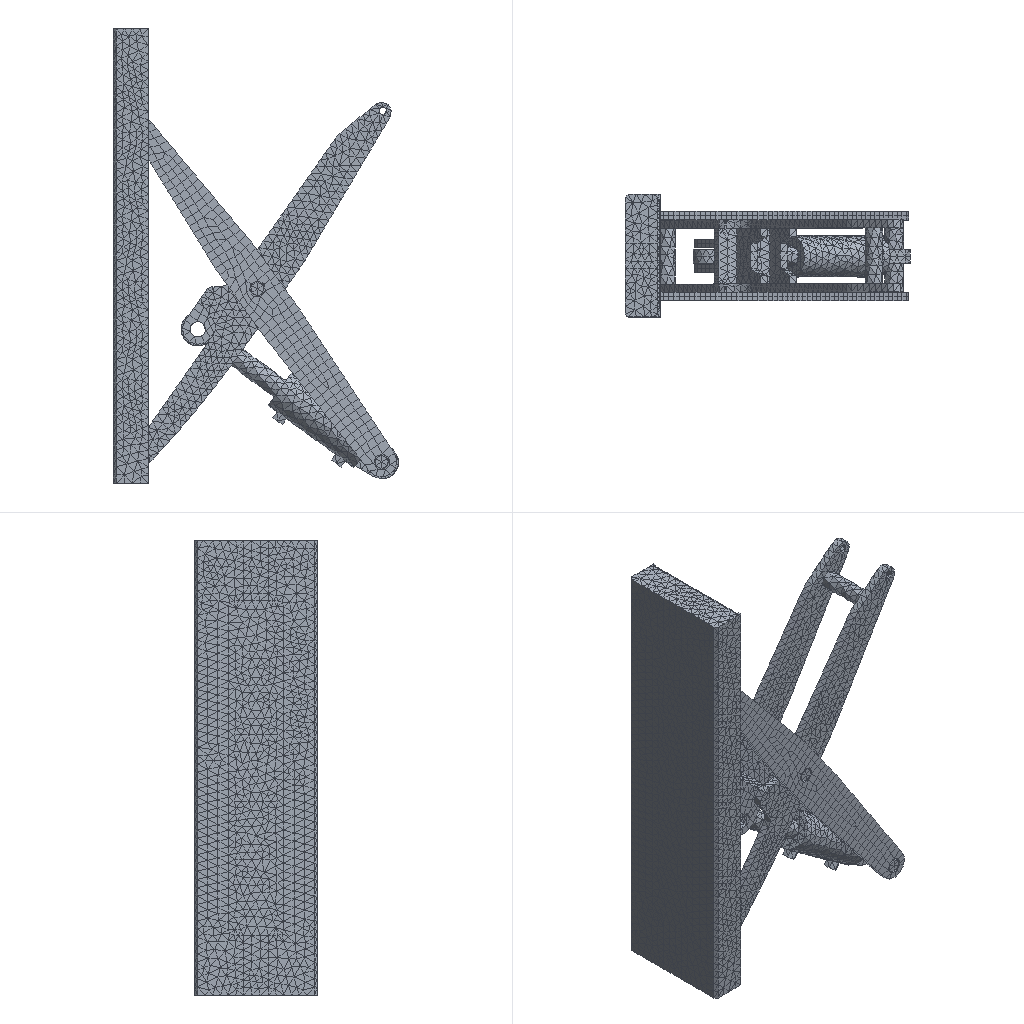Simulation study | ansys workbench
Set-up summary:
category,name,step,type,value,unit,region
solver,ansys_mapdl
solver,version,,,20.2
units,MPA,,stated
analysis,deck,,transient,transient
load_step,requested,,,2
analysis,nlgeom,,,True
mesh,nodes,,,10198
mesh,elements,,,28619
element_type,ANSYS 185 (type 1),,solid,12454
element_type,ANSYS 185 (type 2),,solid,5961
element_type,ANSYS 185 (type 3),,solid,52
element_type,ANSYS 185 (type 4),,solid,52
element_type,ANSYS 185 (type 5),,solid,490
element_type,ANSYS 185 (type 6),,solid,490
element_type,ANSYS 185 (type 7),,solid,1736
element_type,ANSYS 185 (type 8),,solid,725
element_type,ANSYS 185 (type 9),,solid,425
element_type,ANSYS 185 (type 10),,solid,1992
element_type,ANSYS 185 (type 11),,solid,1163
element_type,ANSYS 154 (type 12),,surface,706
element_type,ANSYS 174 (type 13),,contact,30
element_type,ANSYS 170 (type 14),,target,0
element_type,ANSYS 174 (type 15),,contact,12
element_type,ANSYS 170 (type 16),,target,0
element_type,ANSYS 174 (type 17),,contact,50
element_type,ANSYS 170 (type 18),,target,0
element_type,ANSYS 174 (type 19),,contact,12
element_type,ANSYS 170 (type 20),,target,0
element_type,ANSYS 174 (type 21),,contact,20
element_type,ANSYS 170 (type 22),,target,0
element_type,ANSYS 174 (type 23),,contact,12
element_type,ANSYS 170 (type 24),,target,0
element_type,ANSYS 174 (type 25),,contact,20
element_type,ANSYS 170 (type 26),,target,0
element_type,ANSYS 174 (type 27),,contact,12
element_type,ANSYS 170 (type 28),,target,0
element_type,ANSYS 174 (type 29),,contact,20
element_type,ANSYS 170 (type 30),,target,0
element_type,ANSYS 174 (type 31),,contact,14
element_type,ANSYS 170 (type 32),,target,0
element_type,ANSYS 174 (type 33),,contact,20
element_type,ANSYS 170 (type 34),,target,0
element_type,ANSYS 174 (type 35),,contact,14
element_type,ANSYS 170 (type 36),,target,0
element_type,ANSYS 174 (type 37),,contact,22
element_type,ANSYS 170 (type 38),,target,0
element_type,ANSYS 174 (type 39),,contact,14
element_type,ANSYS 170 (type 40),,target,0
element_type,ANSYS 174 (type 41),,contact,22
element_type,ANSYS 170 (type 42),,target,0
element_type,ANSYS 174 (type 43),,contact,14
element_type,ANSYS 170 (type 44),,target,0
element_type,ANSYS 174 (type 45),,contact,24
element_type,ANSYS 170 (type 46),,target,0
element_type,ANSYS 174 (type 47),,contact,28
element_type,ANSYS 170 (type 48),,target,0
element_type,ANSYS 174 (type 49),,contact,52
element_type,ANSYS 170 (type 50),,target,0
element_type,ANSYS 174 (type 51),,contact,334
element_type,ANSYS 170 (type 52),,target,0
element_type,ANSYS 174 (type 53),,contact,32
element_type,ANSYS 170 (type 54),,target,0
element_type,ANSYS 174 (type 55),,contact,56
element_type,ANSYS 170 (type 56),,target,0
element_type,ANSYS 174 (type 57),,contact,104
element_type,ANSYS 170 (type 58),,target,0
element_type,ANSYS 174 (type 59),,contact,56
element_type,ANSYS 170 (type 60),,target,0
element_type,ANSYS 174 (type 61),,contact,116
element_type,ANSYS 170 (type 62),,target,0
element_type,ANSYS 174 (type 63),,contact,1037
element_type,ANSYS 170 (type 64),,target,0
element_type,ANSYS 174 (type 65),,contact,32
element_type,ANSYS 170 (type 66),,target,0
element_type,ANSYS 174 (type 67),,contact,122
element_type,ANSYS 170 (type 68),,target,0
element_type,ANSYS 174 (type 69),,contact,28
element_type,ANSYS 170 (type 70),,target,0
element_type,ANSYS 174 (type 71),,contact,28
element_type,ANSYS 170 (type 72),,target,0
element_type,ANSYS 184 (type 73),,mpc,1
element_type,ANSYS 184 (type 74),,mpc,1
element_type,ANSYS 184 (type 75),,mpc,1
element_type,ANSYS 184 (type 76),,mpc,1
element_type,ANSYS 184 (type 77),,mpc,1
element_type,ANSYS 184 (type 78),,mpc,1
element_type,ANSYS 184 (type 79),,mpc,1
element_type,ANSYS 184 (type 80),,mpc,1
element_type,ANSYS 184 (type 81),,mpc,1
element_type,ANSYS 184 (type 82),,mpc,1
element_type,ANSYS 184 (type 83),,mpc,1
element_type,ANSYS 184 (type 84),,mpc,1
element_type,ANSYS 184 (type 85),,mpc,1
element_type,ANSYS 184 (type 86),,mpc,1
element_type,ANSYS 184 (type 87),,mpc,1
element_type,ANSYS 184 (type 88),,mpc,1
load,load commands in deck,,count,4
bc,support commands in deck,,count,1
named_set,_ELMISC,,component
material,1,,in results
material,2,,in results
material,3,,in results
material,4,,in results
material,5,,in results
material,6,,in results
material,7,,in results
material,8,,in results
material,9,,in results
material,10,,in results
material,11,,in results
check,setup vs results,,match,"results also hold 0 node(s) and 30 element(s) the deck makes with ['EN']; those were not compared; 2 setup node(s) no element uses are not in the results (e.g. [10272, 10274]); 78 node(s) the solver created internally for pilot nodes (solve.out) are in the results only; 706 surface effect element(s) are not in the reader's mesh and were not compared"
Ansys APDL input file, long lists of numbers shortened:
/batch
/config,noeldb,1     ! force off writing results to database
*get,_wallstrt,active,,time,wall
! ANSYS input file written by Workbench version 2020 R2
! File used for geometry attach: E:\LINSHIWENJIAN\WB_DESKTOP-V417B2O_Adminis_37620_2\unsaved_project_files\dp0\Geom\DM\Geom.scdoc
/title,___st--__ (B5)
*DIM,_wb_ProjectScratch_dir,string,248
_wb_ProjectScratch_dir(1) = 'E:\_ProjectScratch\ScrF0D5\'
*DIM,_wb_SolverFiles_dir,string,248
_wb_SolverFiles_dir(1) = 'E:\升降台st_files\dp0\SYS-1\MECH\'
*DIM,_wb_userfiles_dir,string,248
_wb_userfiles_dir(1) = 'E:\升降台st_files\user_files\'
/com,--- Data in consistent NMM units. See Solving Units in the help system for more information.
/units,MPA
/nopr
/wb,file,start              !  signify a WB generated input file
/prep7
! Turn off shape checking because checks already performed inside WB mesher.
! See help system for more information.
SHPP,OFF,,NOWARN
/nolist
etcon,set             ! allow ANSYS to choose best KEYOP's for 180x elements
/com,*********** Nodes for the whole assembly ***********
nblock,3,,11182
(1i9,3e20.9e3)
        1    -5.667923198E+02    -1.150000000E+02     5.191691898E+02
! (10165 more lines like these left out)
-1
/com,*********** Nodes for all Remote Points ***********
nblock,3
(1i9,3e20.9e3)
    10244    -8.508159903E+02    -3.149998116E+01     1.243113147E+03
! (31 more lines like these left out)
-1
/wb,elem,start            !  set before creation of elements
/com,*********** Elements for Body 1 "____\____5" ***********
et,1,185
eblock,19,solid,,12454
(19i9)
        1        1        1        1        0        0        0        0        8        0    12107     5574     8263     8237     8237     8258     8258     8258     8258
! (12453 more lines like these left out)
-1
/com,*********** Elements for Body 2 "______1\____-____9" ***********
et,2,185
eblock,19,solid,,5961
(19i9)
        2        2        2        2        0        0        0        0        8        0     6146     2654     2655     2896     2896     4170     4170     4170     4170
! (5960 more lines like these left out)
-1
/com,*********** Elements for Body 3 "______1\____-____4[2]" ***********
et,3,185
eblock,19,solid,,52
(19i9)
        3        3        3        3        0        0        0        0        8        0     3377     1207     1213     1269     1268     1220     1214     1277     1276
! (51 more lines like these left out)
-1
/com,*********** Elements for Body 4 "______1\____-____4[1]" ***********
et,4,185
eblock,19,solid,,52
(19i9)
        4        4        4        4        0        0        0        0        8        0        1        3        9       65       64       16       10       69       70
! (51 more lines like these left out)
-1
/com,*********** Elements for Body 5 "______2-2\____-____1" ***********
et,5,185
eblock,19,solid,,490
(19i9)
        5        5        5        5        0        0        0        0        8        0    24561     8325     8494     8376     8483     8670     8501     8619     8512
! (489 more lines like these left out)
-1
/com,*********** Elements for Body 6 "______2-2\____-____1" ***********
et,6,185
eblock,19,solid,,490
(19i9)
        6        6        6        6        0        0        0        0        8        0    25051     9246     9415     9297     9404     9591     9422     9540     9433
! (489 more lines like these left out)
-1
/com,*********** Elements for Body 7 "________\M27 ______1" ***********
et,7,185
eblock,19,solid,,1736
(19i9)
        7        7        7        7        0        0        0        0        8        0      478      387      466      865      865      859      859      859      859
! (1735 more lines like these left out)
-1
/com,*********** Elements for Body 8 "________-4\____-____4" ***********
et,8,185
eblock,19,solid,,725
(19i9)
        8        8        8        8        0        0        0        0        8        0     3429     1336     1516     1518     1518     1576     1576     1576     1576
! (724 more lines like these left out)
-1
/com,*********** Elements for Body 9 "____3\____-____1" ***********
et,9,185
eblock,19,solid,,425
(19i9)
        9        9        9        9        0        0        0        0        8        0       53      154      204      275      275      161      161      161      161
! (424 more lines like these left out)
-1
/com,*********** Elements for Body 10 "Geom\____3" ***********
et,10,185
eblock,19,solid,,1992
(19i9)
       10       10       10       10        0        0        0        0        8        0     4154     1729     2127     1988     1988     1989     1989     1989     1989
! (1991 more lines like these left out)
-1
/com,*********** Elements for Body 11 "Geom\____3" ***********
et,11,185
eblock,19,solid,,1163
(19i9)
       11       11       11       11        0        0        0        0        8        0     2214      902      944     1193     1193     1192     1192     1192     1192
! (1162 more lines like these left out)
-1
/wb,elem,end               !  done creating elements
/com,*********** Send User Defined Coordinate System(s) ***********
local,12,0,-850.816,-31.5,1243.113,0.,-90.,0.
local,13,0,-850.816,-288.465,1243.113,0.,90.,0.
local,14,0,-850.816,-45.,-15.415,0.,90.,0.
local,15,0,-850.816,-275.,-15.415,0.,90.,0.
local,16,0,-404.145,-305.,621.427,0.,90.,0.
local,17,0,-404.145,-15.,621.427,0.,-90.,0.
local,18,0,42.339,-15.,0.,0.,-90.,0.
local,19,0,42.339,-305.,0.,0.,-90.,0.
local,20,0,42.339,-160.,0.,0.,-90.,0.
local,21,0,-298.045,-160.,245.696,-4.58105518942482e-030,-3.30668626972939e-030,-144.178
local,22,0,-850.816,18.,1243.113,90.,-4.2964952914991e-031,-90.
local,23,0,-850.816,-337.501,1243.113,-90.,-4.2964952914991e-031,-90.
local,24,0,42.339,-160.,0.,0.,90.,0.
local,25,0,-910.816,-160.,947.28,0.,0.,0.
local,26,0,-520.078,-160.,556.037,0.,0.,25.036
local,27,0,-618.325,-160.,476.879,7.934914251054e-022,-90.,3.35337834212987e-014
csys,0
toffst,273.15,  ! Temperature offset from absolute zero
/com,*********** Set Reference Temperature ***********
tref,22.
/wb,mat,start              !  starting to send materials
/com,*********** Send Materials ***********
MP,DENS,1,7.8e-09,	! tonne mm^-3
MP,EX,1,210000,	! tonne s^-2 mm^-1
MP,NUXY,1,0.3,
MP,DENS,2,7.8e-09,	! tonne mm^-3
! (29 more lines like these left out)
/wb,mat,end                !  done sending materials
!************************* Model Summary ********************
!____\____5,	1,	matid,	1
!______1\____-____9,	1,	matid,	2
!______1\____-____4[2],	1,	matid,	3
!______1\____-____4[1],	1,	matid,	4
!______2-2\____-____1,	1,	matid,	5
!______2-2\____-____1,	1,	matid,	6
!________\M27 ______1,	1,	matid,	7
!________-4\____-____4,	1,	matid,	8
!____3\____-____1,	1,	matid,	9
!Geom\____3,	1,	matid,	10
!Geom\____3,	1,	matid,	11
!************************* End Model Summary ********************
! get the diagonal of the bounding box. Needed later for other things
*get,_xmin,node,,mnloc,x
*get,_ymin,node,,mnloc,y
*get,_zmin,node,,mnloc,z
*get,_xmax,node,,mxloc,x
*get,_ymax,node,,mxloc,y
*get,_zmax,node,,mxloc,z
_ASMDIAG=(_xmax-_xmin)*(_xmax-_xmin)+(_ymax-_ymin)*(_ymax-_ymin)+(_zmax-_zmin)*(_zmax-_zmin)
_ASMDIAG=SQRT(_ASMDIAG)
/wb,contact,start          !  starting to send contact
/wb,contact,end            !  done creating contacts
/golist
/wb,load,start             !  starting to send loads
/com,*********** Define Force Using Surface Effect Elements ***********
local,28,0,0.,0.,0.,0.,0.,0.
csys,0
et,12,154
eblock,10,,,706
(15i9)
    42543       12       12       12       28     7893     7898     7894     7894
! (705 more lines like these left out)
-1
esel,s,type,,12
keyop,12,2,1                ! Apply load in local coordinate system
keyop,12,7,1                ! Use original area so load is constant in large deformation
keyop,12,11,2               ! Use real and not project area
esel,all
/com,*********** Create Remote Point "内部远程点" ***********
! -------- Remote Point Used by "回转 - Geom\____3 至 ______2-2\____-____1" --------
*set,tid,14
*set,cid,13
et,cid,174
et,tid,170
keyo,tid,2,1               ! Don't fix the pilot node
keyo,tid,4,0               ! Activate all DOF's due to large deformation
keyo,cid,12,5              ! Bonded Contact
keyo,cid,4,2               ! Rigid CERIG style load
keyo,cid,2,2               ! MPC style contact
eblock,10,,,30
(15i9)
    43249       13       13       13        0      867      866     1074     1074
! (29 more lines like these left out)
-1
*set,_npilot,10244
_npilot115=_npilot
type,tid
mat ,cid
real,cid
tshape,pilo
en,43279,_npilot
tshape
csys,12
nrot,10244
csys,0
/com,*********** Create Remote Point "内部远程点 2" ***********
! -------- Remote Point Used by "回转 - Geom\____3 至 ______2-2\____-____1" --------
*set,tid,16
*set,cid,15
et,cid,174
et,tid,170
keyo,tid,2,1               ! Don't fix the pilot node
keyo,tid,4,0               ! Activate all DOF's due to large deformation
keyo,cid,12,5              ! Bonded Contact
keyo,cid,4,2               ! Rigid CERIG style load
keyo,cid,2,2               ! MPC style contact
eblock,10,,,12
(15i9)
    43280       15       15       15        0     9006     9012     8962     8958
! (11 more lines like these left out)
-1
*set,_npilot,10245
_npilot116=_npilot
type,tid
mat ,cid
real,cid
tshape,pilo
en,43292,_npilot
tshape
csys,12
nrot,10245
csys,0
/com,*********** Create Remote Point "内部远程点 3" ***********
! -------- Remote Point Used by "回转 - Geom\____3 至 ______2-2\____-____1" --------
*set,tid,18
*set,cid,17
et,cid,174
et,tid,170
keyo,tid,2,1               ! Don't fix the pilot node
keyo,tid,4,0               ! Activate all DOF's due to large deformation
keyo,cid,12,5              ! Bonded Contact
keyo,cid,4,2               ! Rigid CERIG style load
keyo,cid,2,2               ! MPC style contact
eblock,10,,,50
(15i9)
    43293       17       17       17        0     1605     1606     1930     1930
! (49 more lines like these left out)
-1
*set,_npilot,10246
_npilot119=_npilot
type,tid
mat ,cid
real,cid
tshape,pilo
en,43343,_npilot
tshape
csys,13
nrot,10246
csys,0
/com,*********** Create Remote Point "内部远程点 4" ***********
! -------- Remote Point Used by "回转 - Geom\____3 至 ______2-2\____-____1" --------
*set,tid,20
*set,cid,19
et,cid,174
et,tid,170
keyo,tid,2,1               ! Don't fix the pilot node
keyo,tid,4,0               ! Activate all DOF's due to large deformation
keyo,cid,12,5              ! Bonded Contact
keyo,cid,4,2               ! Rigid CERIG style load
keyo,cid,2,2               ! MPC style contact
eblock,10,,,12
(15i9)
    43344       19       19       19        0     9927     9933     9883     9879
! (11 more lines like these left out)
-1
*set,_npilot,10247
_npilot120=_npilot
type,tid
mat ,cid
real,cid
tshape,pilo
en,43356,_npilot
tshape
csys,13
nrot,10247
csys,0
/com,*********** Create Remote Point "内部远程点 5" ***********
! -------- Remote Point Used by "回转 - ______1\____-____9 至 ____\____5" --------
*set,tid,22
*set,cid,21
et,cid,174
et,tid,170
keyo,tid,2,1               ! Don't fix the pilot node
keyo,tid,4,0               ! Activate all DOF's due to large deformation
keyo,cid,12,5              ! Bonded Contact
keyo,cid,4,2               ! Rigid CERIG style load
keyo,cid,2,2               ! MPC style contact
eblock,10,,,20
(15i9)
    43357       21       21       21        0     2212     2211     3540     3540
! (19 more lines like these left out)
-1
*set,_npilot,10248
_npilot123=_npilot
type,tid
mat ,cid
real,cid
tshape,pilo
en,43377,_npilot
tshape
csys,14
nrot,10248
csys,0
/com,*********** Create Remote Point "内部远程点 6" ***********
! -------- Remote Point Used by "回转 - ______1\____-____9 至 ____\____5" --------
*set,tid,24
*set,cid,23
et,cid,174
et,tid,170
keyo,tid,2,1               ! Don't fix the pilot node
keyo,tid,4,0               ! Activate all DOF's due to large deformation
keyo,cid,12,5              ! Bonded Contact
keyo,cid,4,2               ! Rigid CERIG style load
keyo,cid,2,2               ! MPC style contact
eblock,10,,,12
(15i9)
    43378       23       23       23        0     4656     4655     4662     4662
! (11 more lines like these left out)
-1
*set,_npilot,10249
_npilot124=_npilot
type,tid
mat ,cid
real,cid
tshape,pilo
en,43390,_npilot
tshape
csys,14
nrot,10249
csys,0
/com,*********** Create Remote Point "内部远程点 7" ***********
! -------- Remote Point Used by "回转 - ______1\____-____9 至 ____\____5" --------
*set,tid,26
*set,cid,25
et,cid,174
et,tid,170
keyo,tid,2,1               ! Don't fix the pilot node
keyo,tid,4,0               ! Activate all DOF's due to large deformation
keyo,cid,12,5              ! Bonded Contact
keyo,cid,4,2               ! Rigid CERIG style load
keyo,cid,2,2               ! MPC style contact
eblock,10,,,20
(15i9)
    43391       25       25       25        0     2249     2244     3527     3527
! (19 more lines like these left out)
-1
*set,_npilot,10250
_npilot127=_npilot
type,tid
mat ,cid
real,cid
tshape,pilo
en,43411,_npilot
tshape
csys,15
nrot,10250
csys,0
/com,*********** Create Remote Point "内部远程点 8" ***********
! -------- Remote Point Used by "回转 - ______1\____-____9 至 ____\____5" --------
*set,tid,28
*set,cid,27
et,cid,174
et,tid,170
keyo,tid,2,1               ! Don't fix the pilot node
keyo,tid,4,0               ! Activate all DOF's due to large deformation
keyo,cid,12,5              ! Bonded Contact
keyo,cid,4,2               ! Rigid CERIG style load
keyo,cid,2,2               ! MPC style contact
eblock,10,,,12
(15i9)
    43412       27       27       27        0     4574     4575     4581     4581
! (11 more lines like these left out)
-1
*set,_npilot,10251
_npilot128=_npilot
type,tid
mat ,cid
real,cid
tshape,pilo
en,43424,_npilot
tshape
csys,15
nrot,10251
csys,0
/com,*********** Create Remote Point "内部远程点 9" ***********
! -------- Remote Point Used by "回转 - ______1\____-____9 至 ______2-2\____-____1" --------
*set,tid,30
*set,cid,29
et,cid,174
et,tid,170
keyo,tid,2,1               ! Don't fix the pilot node
keyo,tid,4,0               ! Activate all DOF's due to large deformation
keyo,cid,12,5              ! Bonded Contact
keyo,cid,4,2               ! Rigid CERIG style load
keyo,cid,2,2               ! MPC style contact
eblock,10,,,20
(15i9)
    43425       29       29       29        0     3530     2235     3531     3531
! (19 more lines like these left out)
-1
*set,_npilot,10252
_npilot131=_npilot
type,tid
mat ,cid
real,cid
tshape,pilo
en,43445,_npilot
tshape
csys,16
nrot,10252
csys,0
/com,*********** Create Remote Point "内部远程点 10" ***********
! -------- Remote Point Used by "回转 - ______1\____-____9 至 ______2-2\____-____1" --------
*set,tid,32
*set,cid,31
et,cid,174
et,tid,170
keyo,tid,2,1               ! Don't fix the pilot node
keyo,tid,4,0               ! Activate all DOF's due to large deformation
keyo,cid,12,5              ! Bonded Contact
keyo,cid,4,2               ! Rigid CERIG style load
keyo,cid,2,2               ! MPC style contact
eblock,10,,,14
(15i9)
    43446       31       31       31        0     9913     9920     9890     9885
! (13 more lines like these left out)
-1
*set,_npilot,10253
_npilot132=_npilot
type,tid
mat ,cid
real,cid
tshape,pilo
en,43460,_npilot
tshape
csys,16
nrot,10253
csys,0
/com,*********** Create Remote Point "内部远程点 13" ***********
! -------- Remote Point Used by "回转 - ______1\____-____9 至 ______2-2\____-____1" --------
*set,tid,34
*set,cid,33
et,cid,174
et,tid,170
keyo,tid,2,1               ! Don't fix the pilot node
keyo,tid,4,0               ! Activate all DOF's due to large deformation
keyo,cid,12,5              ! Bonded Contact
keyo,cid,4,2               ! Rigid CERIG style load
keyo,cid,2,2               ! MPC style contact
eblock,10,,,20
(15i9)
    43461       33       33       33        0     2197     3541     2198     2198
! (19 more lines like these left out)
-1
*set,_npilot,10256
_npilot139=_npilot
type,tid
mat ,cid
real,cid
tshape,pilo
en,43481,_npilot
tshape
csys,17
nrot,10256
csys,0
/com,*********** Create Remote Point "内部远程点 14" ***********
! -------- Remote Point Used by "回转 - ______1\____-____9 至 ______2-2\____-____1" --------
*set,tid,36
*set,cid,35
et,cid,174
et,tid,170
keyo,tid,2,1               ! Don't fix the pilot node
keyo,tid,4,0               ! Activate all DOF's due to large deformation
keyo,cid,12,5              ! Bonded Contact
keyo,cid,4,2               ! Rigid CERIG style load
keyo,cid,2,2               ! MPC style contact
eblock,10,,,14
(15i9)
    43482       35       35       35        0     8992     8999     8969     8964
! (13 more lines like these left out)
-1
*set,_npilot,10257
_npilot140=_npilot
type,tid
mat ,cid
real,cid
tshape,pilo
en,43496,_npilot
tshape
csys,17
nrot,10257
csys,0
/com,*********** Create Remote Point "内部远程点 17" ***********
! -------- Remote Point Used by "回转 - ____3\____-____1 至 ______2-2\____-____1" --------
*set,tid,38
*set,cid,37
et,cid,174
et,tid,170
keyo,tid,2,1               ! Don't fix the pilot node
keyo,tid,4,0               ! Activate all DOF's due to large deformation
keyo,cid,12,5              ! Bonded Contact
keyo,cid,4,2               ! Rigid CERIG style load
keyo,cid,2,2               ! MPC style contact
eblock,10,,,22
(15i9)
    43497       37       37       37        0      175      176      197      197
! (21 more lines like these left out)
-1
*set,_npilot,10260
_npilot147=_npilot
type,tid
mat ,cid
real,cid
tshape,pilo
en,43519,_npilot
tshape
csys,18
nrot,10260
csys,0
/com,*********** Create Remote Point "内部远程点 18" ***********
! -------- Remote Point Used by "回转 - ____3\____-____1 至 ______2-2\____-____1" --------
*set,tid,40
*set,cid,39
et,cid,174
et,tid,170
keyo,tid,2,1               ! Don't fix the pilot node
keyo,tid,4,0               ! Activate all DOF's due to large deformation
keyo,cid,12,5              ! Bonded Contact
keyo,cid,4,2               ! Rigid CERIG style load
keyo,cid,2,2               ! MPC style contact
eblock,10,,,14
(15i9)
    43520       39       39       39        0     8978     8985     8976     8971
! (13 more lines like these left out)
-1
*set,_npilot,10261
_npilot148=_npilot
type,tid
mat ,cid
real,cid
tshape,pilo
en,43534,_npilot
tshape
csys,18
nrot,10261
csys,0
/com,*********** Create Remote Point "内部远程点 19" ***********
! -------- Remote Point Used by "回转 - ____3\____-____1 至 ______2-2\____-____1" --------
*set,tid,42
*set,cid,41
et,cid,174
et,tid,170
keyo,tid,2,1               ! Don't fix the pilot node
keyo,tid,4,0               ! Activate all DOF's due to large deformation
keyo,cid,12,5              ! Bonded Contact
keyo,cid,4,2               ! Rigid CERIG style load
keyo,cid,2,2               ! MPC style contact
eblock,10,,,22
(15i9)
    43535       41       41       41        0      141      142      192      192
! (21 more lines like these left out)
-1
*set,_npilot,10262
_npilot151=_npilot
type,tid
mat ,cid
real,cid
tshape,pilo
en,43557,_npilot
tshape
csys,19
nrot,10262
csys,0
/com,*********** Create Remote Point "内部远程点 20" ***********
! -------- Remote Point Used by "回转 - ____3\____-____1 至 ______2-2\____-____1" --------
*set,tid,44
*set,cid,43
et,cid,174
et,tid,170
keyo,tid,2,1               ! Don't fix the pilot node
keyo,tid,4,0               ! Activate all DOF's due to large deformation
keyo,cid,12,5              ! Bonded Contact
keyo,cid,4,2               ! Rigid CERIG style load
keyo,cid,2,2               ! MPC style contact
eblock,10,,,14
(15i9)
    43558       43       43       43        0     9899     9906     9897     9892
! (13 more lines like these left out)
-1
*set,_npilot,10263
_npilot152=_npilot
type,tid
mat ,cid
real,cid
tshape,pilo
en,43572,_npilot
tshape
csys,19
nrot,10263
csys,0
/com,*********** Create Remote Point "内部远程点 21" ***********
! -------- Remote Point Used by "回转 - ____3\____-____1 至 ________\M27 ______1" --------
*set,tid,46
*set,cid,45
et,cid,174
et,tid,170
keyo,tid,2,1               ! Don't fix the pilot node
keyo,tid,4,0               ! Activate all DOF's due to large deformation
keyo,cid,12,5              ! Bonded Contact
keyo,cid,4,2               ! Rigid CERIG style load
keyo,cid,2,2               ! MPC style contact
eblock,10,,,24
(15i9)
    43573       45       45       45        0      149      150      224      224
! (23 more lines like these left out)
-1
*set,_npilot,10264
_npilot195=_npilot
type,tid
mat ,cid
real,cid
tshape,pilo
en,43597,_npilot
tshape
csys,20
nrot,10264
csys,0
/com,*********** Create Remote Point "内部远程点 22" ***********
! -------- Remote Point Used by "回转 - ____3\____-____1 至 ________\M27 ______1" --------
*set,tid,48
*set,cid,47
et,cid,174
et,tid,170
keyo,tid,2,1               ! Don't fix the pilot node
keyo,tid,4,0               ! Activate all DOF's due to large deformation
keyo,cid,12,5              ! Bonded Contact
keyo,cid,4,2               ! Rigid CERIG style load
keyo,cid,2,2               ! MPC style contact
eblock,10,,,28
(15i9)
    43598       47       47       47        0      367      368      803      803
! (27 more lines like these left out)
-1
*set,_npilot,10265
_npilot196=_npilot
type,tid
mat ,cid
real,cid
tshape,pilo
en,43626,_npilot
tshape
csys,20
nrot,10265
csys,0
/com,*********** Create Remote Point "内部远程点 23" ***********
! -------- Remote Point Used by "平移的 - ________-4\____-____4 至 ________\M27 ______1" --------
*set,tid,50
*set,cid,49
et,cid,174
et,tid,170
keyo,tid,2,1               ! Don't fix the pilot node
keyo,tid,4,0               ! Activate all DOF's due to large deformation
keyo,cid,12,5              ! Bonded Contact
keyo,cid,4,2               ! Rigid CERIG style load
keyo,cid,2,2               ! MPC style contact
eblock,10,,,52
(15i9)
    43627       49       49       49        0     1396     1395     1431     1431
! (51 more lines like these left out)
-1
*set,_npilot,10266
_npilot203=_npilot
type,tid
mat ,cid
real,cid
tshape,pilo
en,43679,_npilot
tshape
csys,21
nrot,10266
csys,0
/com,*********** Create Remote Point "内部远程点 24" ***********
! -------- Remote Point Used by "平移的 - ________-4\____-____4 至 ________\M27 ______1" --------
*set,tid,52
*set,cid,51
et,cid,174
et,tid,170
keyo,tid,2,1               ! Don't fix the pilot node
keyo,tid,4,0               ! Activate all DOF's due to large deformation
keyo,cid,12,5              ! Bonded Contact
keyo,cid,4,2               ! Rigid CERIG style load
keyo,cid,2,2               ! MPC style contact
eblock,10,,,334
(15i9)
    43680       51       51       51        0      283      284      666      666
! (333 more lines like these left out)
-1
*set,_npilot,10267
_npilot204=_npilot
type,tid
mat ,cid
real,cid
tshape,pilo
en,44014,_npilot
tshape
csys,21
nrot,10267
csys,0
/com,*********** Create Remote Point "内部远程点 25" ***********
! -------- Remote Point Used by "平移的 - Geom\____3 至 ____\____5" --------
*set,tid,54
*set,cid,53
et,cid,174
et,tid,170
keyo,tid,2,1               ! Don't fix the pilot node
keyo,tid,4,0               ! Activate all DOF's due to large deformation
keyo,cid,12,5              ! Bonded Contact
keyo,cid,4,2               ! Rigid CERIG style load
keyo,cid,2,2               ! MPC style contact
eblock,10,,,32
(15i9)
    44015       53       53       53        0      888      889     1068     1068
! (31 more lines like these left out)
-1
*set,_npilot,10268
_npilot207=_npilot
type,tid
mat ,cid
real,cid
tshape,pilo
en,44047,_npilot
tshape
csys,22
nrot,10268
csys,0
/com,*********** Create Remote Point "内部远程点 26" ***********
! -------- Remote Point Used by "平移的 - Geom\____3 至 ____\____5" --------
*set,tid,56
*set,cid,55
et,cid,174
et,tid,170
keyo,tid,2,1               ! Don't fix the pilot node
keyo,tid,4,0               ! Activate all DOF's due to large deformation
keyo,cid,12,5              ! Bonded Contact
keyo,cid,4,2               ! Rigid CERIG style load
keyo,cid,2,2               ! MPC style contact
eblock,10,,,56
(15i9)
    44048       55       55       55        0     4736     7944     4737     4737
! (55 more lines like these left out)
-1
*set,_npilot,10269
_npilot208=_npilot
type,tid
mat ,cid
real,cid
tshape,pilo
en,44104,_npilot
tshape
csys,22
nrot,10269
csys,0
/com,*********** Create Remote Point "内部远程点 27" ***********
! -------- Remote Point Used by "平移的 - Geom\____3 至 ____\____5" --------
*set,tid,58
*set,cid,57
et,cid,174
et,tid,170
keyo,tid,2,1               ! Don't fix the pilot node
keyo,tid,4,0               ! Activate all DOF's due to large deformation
keyo,cid,12,5              ! Bonded Contact
keyo,cid,4,2               ! Rigid CERIG style load
keyo,cid,2,2               ! MPC style contact
eblock,10,,,104
(15i9)
    44105       57       57       57        0     1593     1947     1989     1989
! (103 more lines like these left out)
-1
*set,_npilot,10270
_npilot211=_npilot
type,tid
mat ,cid
real,cid
tshape,pilo
en,44209,_npilot
tshape
csys,23
nrot,10270
csys,0
/com,*********** Create Remote Point "内部远程点 28" ***********
! -------- Remote Point Used by "平移的 - Geom\____3 至 ____\____5" --------
*set,tid,60
*set,cid,59
et,cid,174
et,tid,170
keyo,tid,2,1               ! Don't fix the pilot node
keyo,tid,4,0               ! Activate all DOF's due to large deformation
keyo,cid,12,5              ! Bonded Contact
keyo,cid,4,2               ! Rigid CERIG style load
keyo,cid,2,2               ! MPC style contact
eblock,10,,,56
(15i9)
    44210       59       59       59        0     4779     4780     7931     7931
! (55 more lines like these left out)
-1
*set,_npilot,10271
_npilot212=_npilot
type,tid
mat ,cid
real,cid
tshape,pilo
en,44266,_npilot
tshape
csys,23
nrot,10271
csys,0
/com,*********** Create Remote Point "内部远程点 30" ***********
! -------- Remote Point Used by "固定的 - 接地 至 ____3\____-____1" --------
*set,tid,62
*set,cid,61
et,cid,174
et,tid,170
keyo,tid,2,1               ! Don't fix the pilot node
keyo,tid,4,0               ! Activate all DOF's due to large deformation
keyo,cid,12,5              ! Bonded Contact
keyo,cid,4,2               ! Rigid CERIG style load
keyo,cid,2,2               ! MPC style contact
eblock,10,,,116
(15i9)
    44267       61       61       61        0      160      159      202      202
! (115 more lines like these left out)
-1
*set,_npilot,10273
_npilot228=_npilot
type,tid
mat ,cid
real,cid
tshape,pilo
en,44383,_npilot
tshape
csys,24
nrot,10273
csys,0
/com,*********** Create Remote Point "内部远程点 32" ***********
! -------- Remote Point Used by "平移的 - 接地 至 ____\____5" --------
*set,tid,64
*set,cid,63
et,cid,174
et,tid,170
keyo,tid,2,1               ! Don't fix the pilot node
keyo,tid,4,0               ! Activate all DOF's due to large deformation
keyo,cid,12,5              ! Bonded Contact
keyo,cid,4,2               ! Rigid CERIG style load
keyo,cid,2,2               ! MPC style contact
eblock,10,,,1037
(15i9)
    44384       63       63       63        0     6746     7155     6876     6876
! (1036 more lines like these left out)
-1
*set,_npilot,10275
_npilot235=_npilot
type,tid
mat ,cid
real,cid
tshape,pilo
en,45421,_npilot
tshape
/com,*********** Create Remote Point "内部远程点 33" ***********
! -------- Remote Point Used by "固定的 - 多个 至 ______1\____-____9" --------
*set,tid,66
*set,cid,65
et,cid,174
et,tid,170
keyo,tid,2,1               ! Don't fix the pilot node
keyo,tid,4,0               ! Activate all DOF's due to large deformation
keyo,cid,12,5              ! Bonded Contact
keyo,cid,4,2               ! Rigid CERIG style load
keyo,cid,2,2               ! MPC style contact
eblock,10,,,32
(15i9)
    45422       65       65       65        0       31      102      100       39
! (31 more lines like these left out)
-1
*set,_npilot,10276
_npilot247=_npilot
type,tid
mat ,cid
real,cid
tshape,pilo
en,45454,_npilot
tshape
csys,26
nrot,10276
csys,0
/com,*********** Create Remote Point "内部远程点 34" ***********
! -------- Remote Point Used by "固定的 - 多个 至 ______1\____-____9" --------
*set,tid,68
*set,cid,67
et,cid,174
et,tid,170
keyo,tid,2,1               ! Don't fix the pilot node
keyo,tid,4,0               ! Activate all DOF's due to large deformation
keyo,cid,12,5              ! Bonded Contact
keyo,cid,4,2               ! Rigid CERIG style load
keyo,cid,2,2               ! MPC style contact
eblock,10,,,122
(15i9)
    45455       67       67       67        0     3838     3849     3854     3854
! (121 more lines like these left out)
-1
*set,_npilot,10277
_npilot248=_npilot
type,tid
mat ,cid
real,cid
tshape,pilo
en,45577,_npilot
tshape
csys,26
nrot,10277
csys,0
/com,*********** Create Remote Point "内部远程点 35" ***********
! -------- Remote Point Used by "回转 - ________-4\____-____4 至 多个" --------
*set,tid,70
*set,cid,69
et,cid,174
et,tid,170
keyo,tid,2,1               ! Don't fix the pilot node
keyo,tid,4,0               ! Activate all DOF's due to large deformation
keyo,cid,12,5              ! Bonded Contact
keyo,cid,4,2               ! Rigid CERIG style load
keyo,cid,2,2               ! MPC style contact
eblock,10,,,28
(15i9)
    45578       69       69       69        0     1333     1334     1517     1517
! (27 more lines like these left out)
-1
*set,_npilot,10278
_npilot279=_npilot
type,tid
mat ,cid
real,cid
tshape,pilo
en,45606,_npilot
tshape
csys,27
nrot,10278
csys,0
/com,*********** Create Remote Point "内部远程点 36" ***********
! -------- Remote Point Used by "回转 - ________-4\____-____4 至 多个" --------
*set,tid,72
*set,cid,71
et,cid,174
et,tid,170
keyo,tid,2,1               ! Don't fix the pilot node
keyo,tid,4,0               ! Activate all DOF's due to large deformation
keyo,cid,12,5              ! Bonded Contact
keyo,cid,4,2               ! Rigid CERIG style load
keyo,cid,2,2               ! MPC style contact
eblock,10,,,28
(15i9)
    45607       71       71       71        0     1264     1272     1271     1270
! (27 more lines like these left out)
-1
*set,_npilot,10279
_npilot280=_npilot
type,tid
mat ,cid
real,cid
tshape,pilo
en,45635,_npilot
tshape
csys,27
nrot,10279
csys,0
/com,*********** Create Joint "回转 - Geom\____3 至 ______2-2\____-____1" ***********
/com,            Real Constant Set For Above Joint Is 73
! Joint Element Type Declaration and Definition using MPC184
*set,_jid,73
et,_jid,184
keyo,_jid,1,6           ! Revolute Joint
keyo,_jid,4,1           ! Z Axis is revolute axis
sectype,_jid, joint, revo, _wbjoint
secjoint,,12,12
mat,_jid
real,_jid
type,_jid
secnum,_jid
en,42489,10244,10245      ! body to body joint
/com,*********** Create Joint "回转 - Geom\____3 至 ______2-2\____-____1" ***********
/com,            Real Constant Set For Above Joint Is 74
! Joint Element Type Declaration and Definition using MPC184
*set,_jid,74
et,_jid,184
keyo,_jid,1,6           ! Revolute Joint
keyo,_jid,4,1           ! Z Axis is revolute axis
sectype,_jid, joint, revo, _wbjoint
secjoint,,13,13
mat,_jid
real,_jid
type,_jid
secnum,_jid
en,42490,10246,10247      ! body to body joint
/com,*********** Create Joint "回转 - ______1\____-____9 至 ____\____5" ***********
/com,            Real Constant Set For Above Joint Is 75
! Joint Element Type Declaration and Definition using MPC184
*set,_jid,75
et,_jid,184
keyo,_jid,1,6           ! Revolute Joint
keyo,_jid,4,1           ! Z Axis is revolute axis
sectype,_jid, joint, revo, _wbjoint
secjoint,,14,14
mat,_jid
real,_jid
type,_jid
secnum,_jid
en,42491,10248,10249      ! body to body joint
/com,*********** Create Joint "回转 - ______1\____-____9 至 ____\____5" ***********
/com,            Real Constant Set For Above Joint Is 76
! Joint Element Type Declaration and Definition using MPC184
*set,_jid,76
et,_jid,184
keyo,_jid,1,6           ! Revolute Joint
keyo,_jid,4,1           ! Z Axis is revolute axis
sectype,_jid, joint, revo, _wbjoint
secjoint,,15,15
mat,_jid
real,_jid
type,_jid
secnum,_jid
en,42492,10250,10251      ! body to body joint
/com,*********** Create Joint "回转 - ______1\____-____9 至 ______2-2\____-____1" ***********
/com,            Real Constant Set For Above Joint Is 77
! Joint Element Type Declaration and Definition using MPC184
*set,_jid,77
et,_jid,184
keyo,_jid,1,6           ! Revolute Joint
keyo,_jid,4,1           ! Z Axis is revolute axis
sectype,_jid, joint, revo, _wbjoint
secjoint,,16,16
mat,_jid
real,_jid
type,_jid
secnum,_jid
en,42493,10252,10253      ! body to body joint
/com,*********** Create Joint "回转 - ______1\____-____9 至 ______2-2\____-____1" ***********
/com,            Real Constant Set For Above Joint Is 78
! Joint Element Type Declaration and Definition using MPC184
*set,_jid,78
et,_jid,184
keyo,_jid,1,6           ! Revolute Joint
keyo,_jid,4,1           ! Z Axis is revolute axis
sectype,_jid, joint, revo, _wbjoint
secjoint,,17,17
mat,_jid
real,_jid
type,_jid
secnum,_jid
en,42495,10256,10257      ! body to body joint
/com,*********** Create Joint "回转 - ____3\____-____1 至 ______2-2\____-____1" ***********
/com,            Real Constant Set For Above Joint Is 79
! Joint Element Type Declaration and Definition using MPC184
*set,_jid,79
et,_jid,184
keyo,_jid,1,6           ! Revolute Joint
keyo,_jid,4,1           ! Z Axis is revolute axis
sectype,_jid, joint, revo, _wbjoint
secjoint,,18,18
mat,_jid
real,_jid
type,_jid
secnum,_jid
en,42497,10260,10261      ! body to body joint
/com,*********** Create Joint "回转 - ____3\____-____1 至 ______2-2\____-____1" ***********
/com,            Real Constant Set For Above Joint Is 80
! Joint Element Type Declaration and Definition using MPC184
*set,_jid,80
et,_jid,184
keyo,_jid,1,6           ! Revolute Joint
keyo,_jid,4,1           ! Z Axis is revolute axis
sectype,_jid, joint, revo, _wbjoint
secjoint,,19,19
mat,_jid
real,_jid
type,_jid
secnum,_jid
en,42498,10262,10263      ! body to body joint
/com,*********** Create Joint "回转 - ____3\____-____1 至 ________\M27 ______1" ***********
/com,            Real Constant Set For Above Joint Is 81
! Joint Element Type Declaration and Definition using MPC184
*set,_jid,81
et,_jid,184
keyo,_jid,1,6           ! Revolute Joint
keyo,_jid,4,1           ! Z Axis is revolute axis
sectype,_jid, joint, revo, _wbjoint
secjoint,,20,20
mat,_jid
real,_jid
type,_jid
secnum,_jid
en,42499,10264,10265      ! body to body joint
/com,*********** Create Joint "平移的 - ________-4\____-____4 至 ________\M27 ______1" ***********
/com,            Real Constant Set For Above Joint Is 82
! Joint Element Type Declaration and Definition using MPC184
*set,_jid,82
et,_jid,184
keyo,_jid,1,10          ! Prismatic Joint
sectype,_jid, joint, pris, _wbjoint
secjoint,,21,21
mat,_jid
real,_jid
type,_jid
secnum,_jid
en,42500,10266,10267      ! body to body joint
/com,*********** Create Joint "平移的 - Geom\____3 至 ____\____5" ***********
/com,            Real Constant Set For Above Joint Is 83
! Joint Element Type Declaration and Definition using MPC184
*set,_jid,83
et,_jid,184
keyo,_jid,1,10          ! Prismatic Joint
sectype,_jid, joint, pris, _wbjoint
secjoint,,22,22
mat,_jid
real,_jid
type,_jid
secnum,_jid
en,42501,10268,10269      ! body to body joint
/com,*********** Create Joint "平移的 - Geom\____3 至 ____\____5" ***********
/com,            Real Constant Set For Above Joint Is 84
! Joint Element Type Declaration and Definition using MPC184
*set,_jid,84
et,_jid,184
keyo,_jid,1,10          ! Prismatic Joint
sectype,_jid, joint, pris, _wbjoint
secjoint,,23,23
mat,_jid
real,_jid
type,_jid
secnum,_jid
en,42502,10270,10271      ! body to body joint
/com,*********** Create Joint "固定的 - 接地 至 ____3\____-____1" ***********
/com,            Real Constant Set For Above Joint Is 85
! Joint Element Type Declaration and Definition using MPC184
*set,_jid,85
et,_jid,184
keyo,_jid,1,13          ! Fixed Joint
sectype,_jid, joint, weld, _wbjoint
secjoint,,24,24
mat,_jid
real,_jid
type,_jid
secnum,_jid
en,42503,,10273        ! body to ground joint
/com,*********** Create Joint "平移的 - 接地 至 ____\____5" ***********
/com,            Real Constant Set For Above Joint Is 86
! Joint Element Type Declaration and Definition using MPC184
*set,_jid,86
et,_jid,184
keyo,_jid,1,10          ! Prismatic Joint
sectype,_jid, joint, pris, _wbjoint
secjoint,,25,25
mat,_jid
real,_jid
type,_jid
secnum,_jid
en,42504,,10275        ! body to ground joint
/com,*********** Create Joint "固定的 - 多个 至 ______1\____-____9" ***********
/com,            Real Constant Set For Above Joint Is 87
! Joint Element Type Declaration and Definition using MPC184
*set,_jid,87
et,_jid,184
keyo,_jid,1,13          ! Fixed Joint
sectype,_jid, joint, weld, _wbjoint
secjoint,,26,26
mat,_jid
real,_jid
type,_jid
secnum,_jid
en,42539,10276,10277      ! body to body joint
/com,*********** Create Joint "回转 - ________-4\____-____4 至 多个" ***********
/com,            Real Constant Set For Above Joint Is 88
! Joint Element Type Declaration and Definition using MPC184
*set,_jid,88
et,_jid,184
keyo,_jid,1,6           ! Revolute Joint
keyo,_jid,4,1           ! Z Axis is revolute axis
sectype,_jid, joint, revo, _wbjoint
secjoint,,27,27
mat,_jid
real,_jid
type,_jid
secnum,_jid
en,42542,10278,10279      ! body to body joint
/com,*********** Create Joint Drivers **********
*DIM,_loadvari287,TABLE,3,1,1,TIME,
! Time values
_loadvari287(1,0,1) = 0.
_loadvari287(2,0,1) = 1.
_loadvari287(3,0,1) = 2.
! Load values
_loadvari287(1,1,1) = 0.
_loadvari287(2,1,1) = 150.
_loadvari287(3,1,1) = 0.
/gst,on,on
fini
*get,_numnode,node,0,count
*get,_numelem,elem,0,count
*get, _MAXELEMNUM, elem, 0, NUM, MAX
*get, _MAXNODENUM, node, 0, NUM, MAX
*get, _MAXELEMTYPE, etyp, 0, NUM, MAX
*get, _MAXREALCONST, real, 0, NUM, MAX
/go
/wb,load,end               !  done creating loads
/com,--- Number of total nodes = %_numnode%
/com,--- Number of contact elements = 3063
/com,--- Number of spring elements = 0
/com,--- Number of bearing elements = 0
/com,--- Number of solid elements = 25540
/com,--- Number of condensed parts = 0
/com,--- Number of total elements = %_numelem%
*get,_wallbsol,active,,time,wall
/com,****************************************************************************
/com,*************************    SOLUTION       ********************************
/com,****************************************************************************
/solu
antype,4                   ! transient analysis
nlgeom,on                  ! Turn on Large Deformation Effects
kbc,1                      ! stepped BC's
_thickRatio=0.364   ! Ratio of thick parts in the model
eqsl,sparse,,,,,1
cntr,print,1               ! print out contact info and also make no initial contact an error
dmpoption,emat,no             ! Don't combine emat file for DANSYS
dmpoption,esav,no             ! Don't combine esav file for DANSYS
trnopt,full,,,,,hht        ! HHT time integration method
tintp, mosp			! Choose transient integration settings for moderate speed application
nldiag,cont,iter           ! print out contact info each equilibrium iteration
rescontrol,define,last,last,,dele	   ! Program Controlled
/com,****************************************************
/com,******************* SOLVE FOR LS 1 OF 2 ****************
esel,s,type,,12
nsle
sfe,all,1,pres,1,0.2516
sfe,all,2,pres,1,0.
sfe,all,3,pres,1,0.
nsel,all
esel,all
/nopr
/gopr
esel,s,type,,82
dj,all,ux,%_loadvari287%
esel,all
autots,on                   ! User turned on automatic time stepping
nsub,30,300,20,OFF
time,1.
timint,on                  ! Turn on time integration effects
outres,erase
outres,all,none
outres,nsol,all,
outres,rsol,all
outres,eangl,all
outres,etmp,all
outres,veng,all
outres,strs,all,
outres,epel,all,
outres,eppl,all,
outres,cont,all,
outres,v,all,
outres,a,all,
/nopr
esel,s,type,,73
esel,a,type,,74,88
cm,_elmisc,elem
esel,all
/gopr
outres,misc,all,_elmisc
! *********** WB SOLVE COMMAND ***********
! check interactive state
*get,ANSINTER_,active,,int
*if,ANSINTER_,ne,0,then
/eof
*endif
solve
/com *************** Write FE CONNECTORS *********
CEWRITE,file,ce,,INTE
/com,****************************************************
/com,*************** FINISHED SOLVE FOR LS 1 *************
/com,****************************************************
/com,******************* SOLVE FOR LS 2 OF 2 ****************
/nopr
/gopr
autots,on                   ! User turned on automatic time stepping
nsub,30,100,20,OFF
time,2.
timint,on                  ! Turn on time integration effects
outres,erase
outres,all,none
outres,nsol,all,
outres,rsol,all
outres,eangl,all
outres,etmp,all
outres,veng,all
outres,strs,all,
outres,epel,all,
outres,eppl,all,
outres,cont,all,
outres,v,all,
outres,a,all,
outres,misc,all,_elmisc
solve
/com,****************************************************
/com,*************** FINISHED SOLVE FOR LS 2 *************
*get,_wallasol,active,,time,wall
/nopr
*get,_numnode,node,0,count
*get,_numelem,elem,0,count
*get, _MAXELEMNUM, elem, 0, NUM, MAX
*get, _MAXNODENUM, node, 0, NUM, MAX,,,INTERNAL
*get, _MAXELEMTYPE, etyp, 0, NUM, MAX
*get, _MAXREALCONST, real, 0, NUM, MAX
/gopr
/post1
xmlo,ENCODING,ISO-8859-1
xmlo,parm
/xml,parm,xml
fini
/gopr
*get,_walldone,active,,time,wall
_preptime=(_wallbsol-_wallstrt)*3600
_solvtime=(_wallasol-_wallbsol)*3600
_posttime=(_walldone-_wallasol)*3600
_totaltim=(_walldone-_wallstrt)*3600
*get,_dlbratio,active,0,solu,dlbr
*get,_combtime,active,0,solu,comb
/com,--- Total number of nodes = %_numnode%
/com,--- Total number of elements = %_numelem%
/com,--- Element load balance ratio = %_dlbratio%
/com,--- Time to combine distributed files = %_combtime%
/wb,file,end               ! done with WB generated input
Results summary:
result,analysis,,,static
result,last_loadstep,,,2
result,primary field,,,displacement
result,reaction total,79,FX,-180921.05,N
result,reaction total,79,FY,0.0,N
result,reaction total,79,FZ,0.0,N
result,mass,,,0.3971,"NMM: mm, ton, N, s, mV, mA, degC"